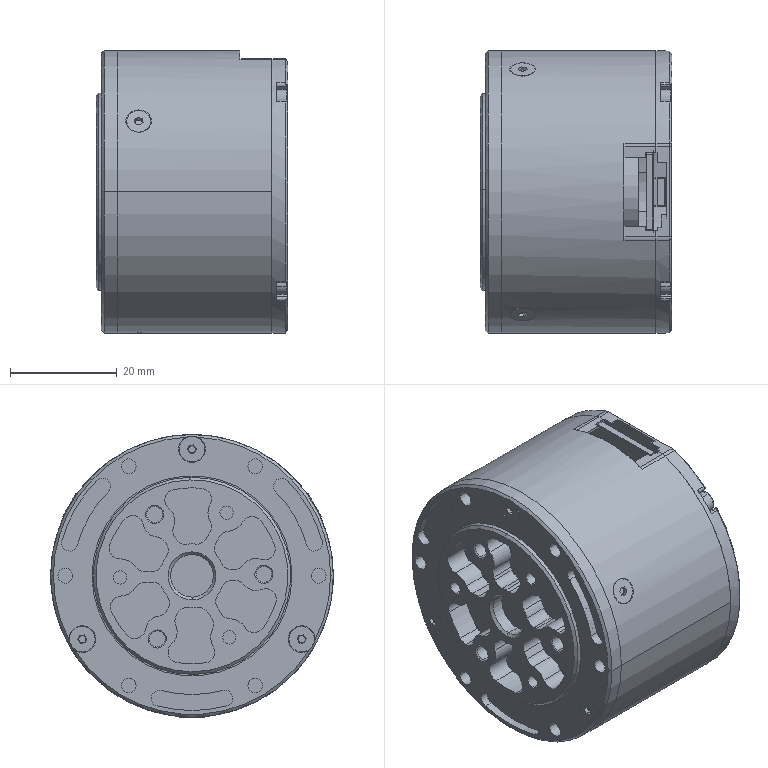Part | SolidWorks | features BaseBody 19 | 19 solids | 1029 faces | box 36 x 53 x 53.058 mm | volume 61188 mm3 | cylinder 485 | plane 332 | cone 136 | spline 76 | commonest cylinder face diameters 4 x140 2.5 x30 3 x25 2.8 x24 1 x18 0.1 x16